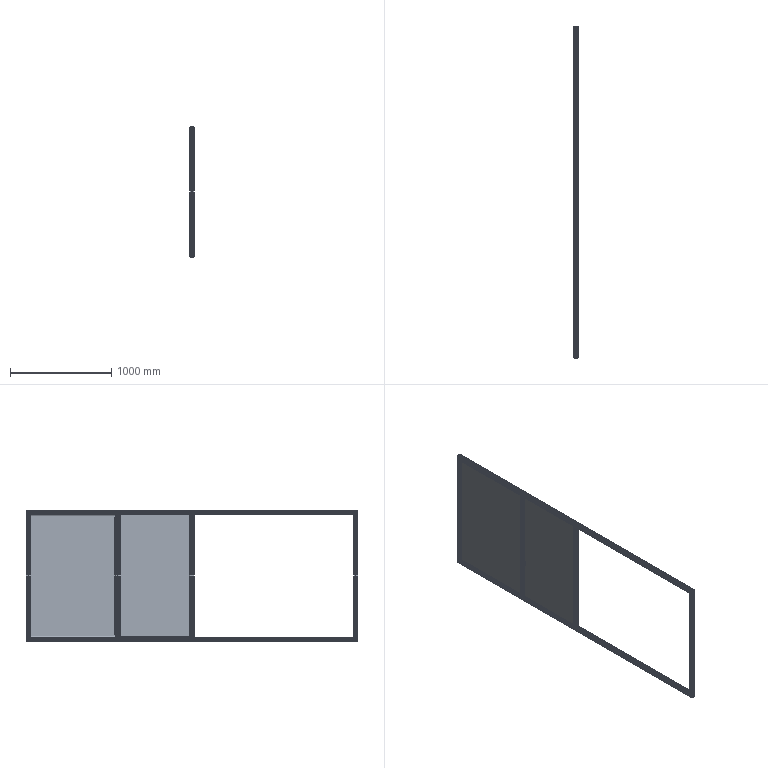Part | SolidWorks | features ReferencePattern 22, LocalLPattern 5, MirrorCompFeat 2, CompositeCurve 1 | 24 solids | 2100 faces | box 40 x 3280 x 1290 mm | volume 16940253 mm3 | plane 1406 | cylinder 694 | commonest cylinder face diameters 6.8 x178 5 x132 2 x68 19 x48 1 x36 6.6 x32